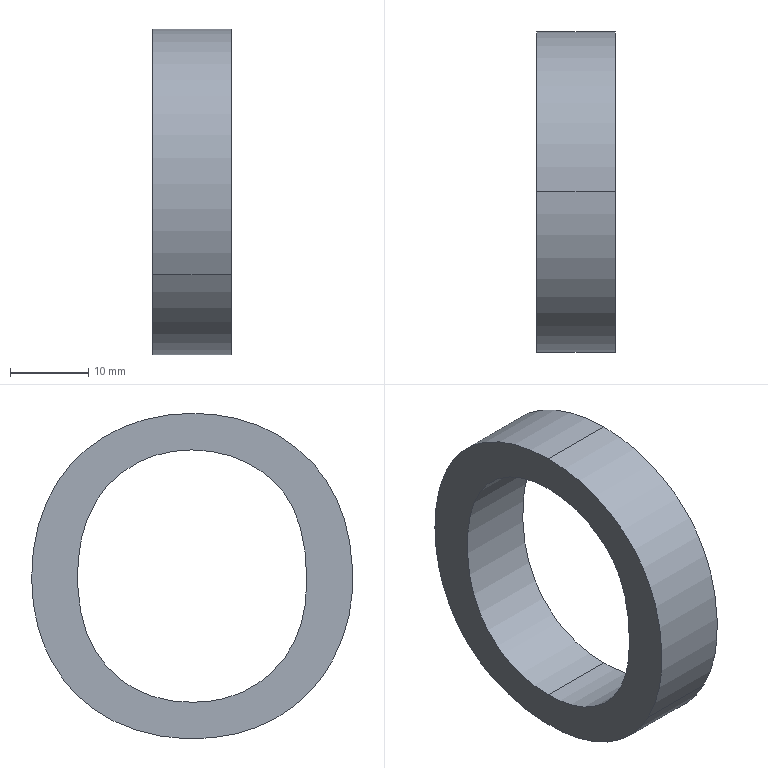Part | NX | features solid 2 | 1 solid | 8 faces | box 10 x 40.994 x 41.56 mm | volume 6055 mm3 | spline 6 | plane 2
STEP:
#1=CARTESIAN_POINT('',(2250.,-504.918,-666.115));
#2=VERTEX_POINT('',#1);
#3=CARTESIAN_POINT('',(2250.,-504.842,-633.885));
#4=VERTEX_POINT('',#3);
#5=CARTESIAN_POINT('',(2250.,-504.918,-666.115));
#6=CARTESIAN_POINT('',(2250.,-500.666,-666.145));
#7=CARTESIAN_POINT('',(2250.,-497.163,-664.769));
#8=CARTESIAN_POINT('',(2250.,-491.648,-659.163));
#9=CARTESIAN_POINT('',(2250.,-490.264,-655.193));
#10=CARTESIAN_POINT('',(2250.,-490.264,-646.826));
#11=CARTESIAN_POINT('',(2250.,-490.83,-643.981));
#12=CARTESIAN_POINT('',(2250.,-492.023,-641.557));
#13=CARTESIAN_POINT('',(2250.,-493.216,-639.132));
#14=CARTESIAN_POINT('',(2250.,-494.945,-637.266));
#15=CARTESIAN_POINT('',(2250.,-497.217,-635.918));
#16=CARTESIAN_POINT('',(2250.,-499.457,-634.589));
#17=CARTESIAN_POINT('',(2250.,-502.027,-633.916));
#18=CARTESIAN_POINT('',(2250.,-504.842,-633.885));
#19=B_SPLINE_CURVE_WITH_KNOTS('',3,(#5,#6,#7,#8,#9,#10,#11,#12,#13,#14,#15,#16,#17,#18),.UNSPECIFIED.,.F.,.F.,(4,2,2,3,3,4),(0.4029,0.5265,0.649,0.7248,0.8038,0.885),.UNSPECIFIED.);
#20=EDGE_CURVE('',#2,#4,#19,.T.);
#21=ORIENTED_EDGE('',*,*,#20,.F.);
#22=CARTESIAN_POINT('',(2260.,-504.918,-666.115));
#23=VERTEX_POINT('',#22);
#24=CARTESIAN_POINT('',(2260.,-504.918,-666.115));
#25=DIRECTION('',(-1.,0.,0.));
#26=VECTOR('',#25,1000.);
#27=LINE('',#24,#26);
#28=EDGE_CURVE('',#23,#2,#27,.T.);
#29=ORIENTED_EDGE('',*,*,#28,.F.);
#30=CARTESIAN_POINT('',(2260.,-504.842,-633.885));
#31=VERTEX_POINT('',#30);
#32=CARTESIAN_POINT('',(2260.,-504.918,-666.115));
#33=CARTESIAN_POINT('',(2260.,-500.666,-666.145));
#34=CARTESIAN_POINT('',(2260.,-497.163,-664.769));
#35=CARTESIAN_POINT('',(2260.,-491.648,-659.163));
#36=CARTESIAN_POINT('',(2260.,-490.264,-655.193));
#37=CARTESIAN_POINT('',(2260.,-490.264,-646.826));
#38=CARTESIAN_POINT('',(2260.,-490.83,-643.981));
#39=CARTESIAN_POINT('',(2260.,-492.023,-641.557));
#40=CARTESIAN_POINT('',(2260.,-493.216,-639.132));
#41=CARTESIAN_POINT('',(2260.,-494.945,-637.266));
#42=CARTESIAN_POINT('',(2260.,-497.217,-635.918));
#43=CARTESIAN_POINT('',(2260.,-499.457,-634.589));
#44=CARTESIAN_POINT('',(2260.,-502.027,-633.916));
#45=CARTESIAN_POINT('',(2260.,-504.842,-633.885));
#46=B_SPLINE_CURVE_WITH_KNOTS('',3,(#32,#33,#34,#35,#36,#37,#38,#39,#40,#41,#42,#43,#44,#45),.UNSPECIFIED.,.F.,.F.,(4,2,2,3,3,4),(0.4029,0.5265,0.649,0.7248,0.8038,0.885),.UNSPECIFIED.);
#47=EDGE_CURVE('',#23,#31,#46,.T.);
#48=ORIENTED_EDGE('',*,*,#47,.T.);
#49=CARTESIAN_POINT('',(2260.,-504.842,-633.885));
#50=DIRECTION('',(-1.,0.,0.));
#51=VECTOR('',#50,1000.);
#52=LINE('',#49,#51);
#53=EDGE_CURVE('',#31,#4,#52,.T.);
#54=ORIENTED_EDGE('',*,*,#53,.T.);
#55=EDGE_LOOP('',(#21,#29,#48,#54));
#56=FACE_BOUND('',#55,.T.);
#57=CARTESIAN_POINT('',(2260.,-504.918,-666.115));
#58=CARTESIAN_POINT('',(2250.,-504.918,-666.115));
#59=CARTESIAN_POINT('',(2260.,-502.844,-666.13));
#60=CARTESIAN_POINT('',(2250.,-502.844,-666.13));
#61=CARTESIAN_POINT('',(2260.,-499.063,-665.494));
#62=CARTESIAN_POINT('',(2250.,-499.063,-665.494));
#63=CARTESIAN_POINT('',(2260.,-495.169,-662.989));
#64=CARTESIAN_POINT('',(2250.,-495.169,-662.989));
#65=CARTESIAN_POINT('',(2260.,-492.683,-659.999));
#66=CARTESIAN_POINT('',(2250.,-492.683,-659.999));
#67=CARTESIAN_POINT('',(2260.,-491.36,-657.341));
#68=CARTESIAN_POINT('',(2250.,-491.36,-657.341));
#69=CARTESIAN_POINT('',(2260.,-490.523,-654.26));
#70=CARTESIAN_POINT('',(2250.,-490.523,-654.26));
#71=CARTESIAN_POINT('',(2260.,-490.187,-650.698));
#72=CARTESIAN_POINT('',(2250.,-490.187,-650.698));
#73=CARTESIAN_POINT('',(2260.,-490.359,-646.885));
#74=CARTESIAN_POINT('',(2250.,-490.359,-646.885));
#75=CARTESIAN_POINT('',(2260.,-491.091,-643.562));
#76=CARTESIAN_POINT('',(2250.,-491.091,-643.562));
#77=CARTESIAN_POINT('',(2260.,-492.412,-640.598));
#78=CARTESIAN_POINT('',(2250.,-492.412,-640.598));
#79=CARTESIAN_POINT('',(2260.,-494.719,-637.465));
#80=CARTESIAN_POINT('',(2250.,-494.719,-637.465));
#81=CARTESIAN_POINT('',(2260.,-498.874,-634.639));
#82=CARTESIAN_POINT('',(2250.,-498.874,-634.639));
#83=CARTESIAN_POINT('',(2260.,-502.752,-633.908));
#84=CARTESIAN_POINT('',(2250.,-502.752,-633.908));
#85=CARTESIAN_POINT('',(2260.,-504.842,-633.885));
#86=CARTESIAN_POINT('',(2250.,-504.842,-633.885));
#87=B_SPLINE_SURFACE_WITH_KNOTS('',3,1,((#57,#58),(#59,#60),(#61,#62),(#63,#64),(#65,#66),(#67,#68),(#69,#70),(#71,#72),(#73,#74),(#75,#76),(#77,#78),(#79,#80),(#81,#82),(#83,#84),(#85,#86)),.SURF_OF_LINEAR_EXTRUSION.,.F.,.F.,.F.,(4,1,1,1,1,1,1,1,1,1,1,1,4),(2,2),(0.4029,0.4632,0.5235,0.5536,0.5837,0.6138,0.644,0.6741,0.7042,0.7344,0.7645,0.8248,0.885),(0.,1.),.UNSPECIFIED.);
#88=ADVANCED_FACE('',(#56),#87,.T.);
#89=CARTESIAN_POINT('',(2250.,-515.191,-637.778));
#90=VERTEX_POINT('',#89);
#91=CARTESIAN_POINT('',(2250.,-504.842,-633.885));
#92=CARTESIAN_POINT('',(2250.,-508.849,-633.916));
#93=CARTESIAN_POINT('',(2250.,-512.291,-635.201));
#94=CARTESIAN_POINT('',(2250.,-515.191,-637.778));
#95=B_SPLINE_CURVE_WITH_KNOTS('',3,(#91,#92,#93,#94),.UNSPECIFIED.,.F.,.F.,(4,4),(0.885,1.),.PIECEWISE_BEZIER_KNOTS.);
#96=EDGE_CURVE('',#4,#90,#95,.T.);
#97=ORIENTED_EDGE('',*,*,#96,.F.);
#98=ORIENTED_EDGE('',*,*,#53,.F.);
#99=CARTESIAN_POINT('',(2260.,-515.191,-637.778));
#100=VERTEX_POINT('',#99);
#101=CARTESIAN_POINT('',(2260.,-504.842,-633.885));
#102=CARTESIAN_POINT('',(2260.,-508.849,-633.916));
#103=CARTESIAN_POINT('',(2260.,-512.291,-635.201));
#104=CARTESIAN_POINT('',(2260.,-515.191,-637.778));
#105=B_SPLINE_CURVE_WITH_KNOTS('',3,(#101,#102,#103,#104),.UNSPECIFIED.,.F.,.F.,(4,4),(0.885,1.),.PIECEWISE_BEZIER_KNOTS.);
#106=EDGE_CURVE('',#31,#100,#105,.T.);
#107=ORIENTED_EDGE('',*,*,#106,.T.);
#108=CARTESIAN_POINT('',(2260.,-515.191,-637.778));
#109=DIRECTION('',(-1.,0.,0.));
#110=VECTOR('',#109,1000.);
#111=LINE('',#108,#110);
#112=EDGE_CURVE('',#100,#90,#111,.T.);
#113=ORIENTED_EDGE('',*,*,#112,.T.);
#114=EDGE_LOOP('',(#97,#98,#107,#113));
#115=FACE_BOUND('',#114,.T.);
#116=CARTESIAN_POINT('',(2260.,-504.842,-633.885));
#117=CARTESIAN_POINT('',(2250.,-504.842,-633.885));
#118=CARTESIAN_POINT('',(2260.,-508.849,-633.916));
#119=CARTESIAN_POINT('',(2250.,-508.849,-633.916));
#120=CARTESIAN_POINT('',(2260.,-512.291,-635.201));
#121=CARTESIAN_POINT('',(2250.,-512.291,-635.201));
#122=CARTESIAN_POINT('',(2260.,-515.191,-637.778));
#123=CARTESIAN_POINT('',(2250.,-515.191,-637.778));
#124=B_SPLINE_SURFACE_WITH_KNOTS('',3,1,((#116,#117),(#118,#119),(#120,#121),(#122,#123)),.SURF_OF_LINEAR_EXTRUSION.,.F.,.F.,.F.,(4,4),(2,2),(0.885,1.),(0.,1.),.PIECEWISE_BEZIER_KNOTS.);
#125=ADVANCED_FACE('',(#115),#124,.T.);
#126=CARTESIAN_POINT('',(2250.,-522.928,-660.588));
#127=VERTEX_POINT('',#126);
#128=CARTESIAN_POINT('',(2250.,-504.872,-629.22));
#129=VERTEX_POINT('',#128);
#130=CARTESIAN_POINT('',(2250.,-522.928,-660.588));
#131=CARTESIAN_POINT('',(2250.,-524.559,-657.426));
#132=CARTESIAN_POINT('',(2250.,-525.4,-654.076));
#133=CARTESIAN_POINT('',(2250.,-525.4,-643.889));
#134=CARTESIAN_POINT('',(2250.,-523.488,-638.688));
#135=CARTESIAN_POINT('',(2250.,-515.855,-631.147));
#136=CARTESIAN_POINT('',(2250.,-510.914,-629.25));
#137=CARTESIAN_POINT('',(2250.,-504.872,-629.22));
#138=B_SPLINE_CURVE_WITH_KNOTS('',3,(#130,#131,#132,#133,#134,#135,#136,#137),.UNSPECIFIED.,.F.,.F.,(4,2,2,4),(0.,0.07116,0.2052,0.3386),.UNSPECIFIED.);
#139=EDGE_CURVE('',#127,#129,#138,.T.);
#140=ORIENTED_EDGE('',*,*,#139,.F.);
#141=CARTESIAN_POINT('',(2260.,-522.928,-660.588));
#142=VERTEX_POINT('',#141);
#143=CARTESIAN_POINT('',(2260.,-522.928,-660.588));
#144=DIRECTION('',(-1.,0.,0.));
#145=VECTOR('',#144,1000.);
#146=LINE('',#143,#145);
#147=EDGE_CURVE('',#142,#127,#146,.T.);
#148=ORIENTED_EDGE('',*,*,#147,.F.);
#149=CARTESIAN_POINT('',(2260.,-504.872,-629.22));
#150=VERTEX_POINT('',#149);
#151=CARTESIAN_POINT('',(2260.,-522.928,-660.588));
#152=CARTESIAN_POINT('',(2260.,-524.559,-657.426));
#153=CARTESIAN_POINT('',(2260.,-525.4,-654.076));
#154=CARTESIAN_POINT('',(2260.,-525.4,-643.889));
#155=CARTESIAN_POINT('',(2260.,-523.488,-638.688));
#156=CARTESIAN_POINT('',(2260.,-515.855,-631.147));
#157=CARTESIAN_POINT('',(2260.,-510.914,-629.25));
#158=CARTESIAN_POINT('',(2260.,-504.872,-629.22));
#159=B_SPLINE_CURVE_WITH_KNOTS('',3,(#151,#152,#153,#154,#155,#156,#157,#158),.UNSPECIFIED.,.F.,.F.,(4,2,2,4),(0.,0.07116,0.2052,0.3386),.UNSPECIFIED.);
#160=EDGE_CURVE('',#142,#150,#159,.T.);
#161=ORIENTED_EDGE('',*,*,#160,.T.);
#162=CARTESIAN_POINT('',(2260.,-504.872,-629.22));
#163=DIRECTION('',(-1.,0.,0.));
#164=VECTOR('',#163,1000.);
#165=LINE('',#162,#164);
#166=EDGE_CURVE('',#150,#129,#165,.T.);
#167=ORIENTED_EDGE('',*,*,#166,.T.);
#168=EDGE_LOOP('',(#140,#148,#161,#167));
#169=FACE_BOUND('',#168,.T.);
#170=CARTESIAN_POINT('',(2260.,-522.928,-660.588));
#171=CARTESIAN_POINT('',(2250.,-522.928,-660.588));
#172=CARTESIAN_POINT('',(2260.,-523.898,-658.707));
#173=CARTESIAN_POINT('',(2250.,-523.898,-658.707));
#174=CARTESIAN_POINT('',(2260.,-524.934,-655.787));
#175=CARTESIAN_POINT('',(2250.,-524.934,-655.787));
#176=CARTESIAN_POINT('',(2260.,-525.444,-651.693));
#177=CARTESIAN_POINT('',(2250.,-525.444,-651.693));
#178=CARTESIAN_POINT('',(2260.,-525.368,-647.482));
#179=CARTESIAN_POINT('',(2250.,-525.368,-647.482));
#180=CARTESIAN_POINT('',(2260.,-524.594,-642.841));
#181=CARTESIAN_POINT('',(2250.,-524.594,-642.841));
#182=CARTESIAN_POINT('',(2260.,-522.526,-638.112));
#183=CARTESIAN_POINT('',(2250.,-522.526,-638.112));
#184=CARTESIAN_POINT('',(2260.,-519.235,-634.2));
#185=CARTESIAN_POINT('',(2250.,-519.235,-634.2));
#186=CARTESIAN_POINT('',(2260.,-513.777,-630.387));
#187=CARTESIAN_POINT('',(2250.,-513.777,-630.387));
#188=CARTESIAN_POINT('',(2260.,-508.705,-629.239));
#189=CARTESIAN_POINT('',(2250.,-508.705,-629.239));
#190=CARTESIAN_POINT('',(2260.,-504.872,-629.22));
#191=CARTESIAN_POINT('',(2250.,-504.872,-629.22));
#192=B_SPLINE_SURFACE_WITH_KNOTS('',3,1,((#170,#171),(#172,#173),(#174,#175),(#176,#177),(#178,#179),(#180,#181),(#182,#183),(#184,#185),(#186,#187),(#188,#189),(#190,#191)),.SURF_OF_LINEAR_EXTRUSION.,.F.,.F.,.F.,(4,1,1,1,1,1,1,1,4),(2,2),(0.,0.04233,0.06349,0.08466,0.127,0.1693,0.2116,0.254,0.3386),(0.,1.),.UNSPECIFIED.);
#193=ADVANCED_FACE('',(#169),#192,.T.);
#194=CARTESIAN_POINT('',(2250.,-487.052,-661.021));
#195=VERTEX_POINT('',#194);
#196=CARTESIAN_POINT('',(2250.,-504.872,-629.22));
#197=CARTESIAN_POINT('',(2250.,-500.895,-629.25));
#198=CARTESIAN_POINT('',(2250.,-497.346,-630.153));
#199=CARTESIAN_POINT('',(2250.,-494.188,-631.911));
#200=CARTESIAN_POINT('',(2250.,-490.998,-633.686));
#201=CARTESIAN_POINT('',(2250.,-488.582,-636.164));
#202=CARTESIAN_POINT('',(2250.,-485.247,-642.497));
#203=CARTESIAN_POINT('',(2250.,-484.406,-646.092));
#204=CARTESIAN_POINT('',(2250.,-484.406,-654.184));
#205=CARTESIAN_POINT('',(2250.,-485.262,-657.824));
#206=CARTESIAN_POINT('',(2250.,-487.052,-661.021));
#207=B_SPLINE_CURVE_WITH_KNOTS('',3,(#196,#197,#198,#199,#200,#201,#202,#203,#204,#205,#206),.UNSPECIFIED.,.F.,.F.,(4,3,2,2,4),(0.3386,0.4247,0.5061,0.5876,0.6712),.UNSPECIFIED.);
#208=EDGE_CURVE('',#129,#195,#207,.T.);
#209=ORIENTED_EDGE('',*,*,#208,.F.);
#210=ORIENTED_EDGE('',*,*,#166,.F.);
#211=CARTESIAN_POINT('',(2260.,-487.052,-661.021));
#212=VERTEX_POINT('',#211);
#213=CARTESIAN_POINT('',(2260.,-504.872,-629.22));
#214=CARTESIAN_POINT('',(2260.,-500.895,-629.25));
#215=CARTESIAN_POINT('',(2260.,-497.346,-630.153));
#216=CARTESIAN_POINT('',(2260.,-494.188,-631.911));
#217=CARTESIAN_POINT('',(2260.,-490.998,-633.686));
#218=CARTESIAN_POINT('',(2260.,-488.582,-636.164));
#219=CARTESIAN_POINT('',(2260.,-485.247,-642.497));
#220=CARTESIAN_POINT('',(2260.,-484.406,-646.092));
#221=CARTESIAN_POINT('',(2260.,-484.406,-654.184));
#222=CARTESIAN_POINT('',(2260.,-485.262,-657.824));
#223=CARTESIAN_POINT('',(2260.,-487.052,-661.021));
#224=B_SPLINE_CURVE_WITH_KNOTS('',3,(#213,#214,#215,#216,#217,#218,#219,#220,#221,#222,#223),.UNSPECIFIED.,.F.,.F.,(4,3,2,2,4),(0.3386,0.4247,0.5061,0.5876,0.6712),.UNSPECIFIED.);
#225=EDGE_CURVE('',#150,#212,#224,.T.);
#226=ORIENTED_EDGE('',*,*,#225,.T.);
#227=CARTESIAN_POINT('',(2260.,-487.052,-661.021));
#228=DIRECTION('',(-1.,0.,0.));
#229=VECTOR('',#228,1000.);
#230=LINE('',#227,#229);
#231=EDGE_CURVE('',#212,#195,#230,.T.);
#232=ORIENTED_EDGE('',*,*,#231,.T.);
#233=EDGE_LOOP('',(#209,#210,#226,#232));
#234=FACE_BOUND('',#233,.T.);
#235=CARTESIAN_POINT('',(2260.,-504.872,-629.22));
#236=CARTESIAN_POINT('',(2250.,-504.872,-629.22));
#237=CARTESIAN_POINT('',(2260.,-502.951,-629.235));
#238=CARTESIAN_POINT('',(2250.,-502.951,-629.235));
#239=CARTESIAN_POINT('',(2260.,-500.223,-629.559));
#240=CARTESIAN_POINT('',(2250.,-500.223,-629.559));
#241=CARTESIAN_POINT('',(2260.,-496.855,-630.609));
#242=CARTESIAN_POINT('',(2250.,-496.855,-630.609));
#243=CARTESIAN_POINT('',(2260.,-494.514,-631.667));
#244=CARTESIAN_POINT('',(2250.,-494.514,-631.667));
#245=CARTESIAN_POINT('',(2260.,-492.139,-633.14));
#246=CARTESIAN_POINT('',(2250.,-492.139,-633.14));
#247=CARTESIAN_POINT('',(2260.,-489.444,-635.44));
#248=CARTESIAN_POINT('',(2250.,-489.444,-635.44));
#249=CARTESIAN_POINT('',(2260.,-486.783,-639.041));
#250=CARTESIAN_POINT('',(2250.,-486.783,-639.041));
#251=CARTESIAN_POINT('',(2260.,-485.152,-643.391));
#252=CARTESIAN_POINT('',(2250.,-485.152,-643.391));
#253=CARTESIAN_POINT('',(2260.,-484.508,-647.139));
#254=CARTESIAN_POINT('',(2250.,-484.508,-647.139));
#255=CARTESIAN_POINT('',(2260.,-484.352,-650.16));
#256=CARTESIAN_POINT('',(2250.,-484.352,-650.16));
#257=CARTESIAN_POINT('',(2260.,-484.519,-653.158));
#258=CARTESIAN_POINT('',(2250.,-484.519,-653.158));
#259=CARTESIAN_POINT('',(2260.,-485.174,-656.88));
#260=CARTESIAN_POINT('',(2250.,-485.174,-656.88));
#261=CARTESIAN_POINT('',(2260.,-486.162,-659.432));
#262=CARTESIAN_POINT('',(2250.,-486.162,-659.432));
#263=CARTESIAN_POINT('',(2260.,-487.052,-661.021));
#264=CARTESIAN_POINT('',(2250.,-487.052,-661.021));
#265=B_SPLINE_SURFACE_WITH_KNOTS('',3,1,((#235,#236),(#237,#238),(#239,#240),(#241,#242),(#243,#244),(#245,#246),(#247,#248),(#249,#250),(#251,#252),(#253,#254),(#255,#256),(#257,#258),(#259,#260),(#261,#262),(#263,#264)),.SURF_OF_LINEAR_EXTRUSION.,.F.,.F.,.F.,(4,1,1,1,1,1,1,1,1,1,1,1,4),(2,2),(0.3386,0.3802,0.401,0.4218,0.4426,0.4634,0.5049,0.5465,0.5673,0.5881,0.6089,0.6296,0.6712),(0.,1.),.UNSPECIFIED.);
#266=ADVANCED_FACE('',(#234),#265,.T.);
#267=CARTESIAN_POINT('',(2250.,-487.052,-661.021));
#268=CARTESIAN_POINT('',(2250.,-488.796,-664.249));
#269=CARTESIAN_POINT('',(2250.,-491.274,-666.681));
#270=CARTESIAN_POINT('',(2250.,-497.717,-669.979));
#271=CARTESIAN_POINT('',(2250.,-501.186,-670.78));
#272=CARTESIAN_POINT('',(2250.,-508.926,-670.78));
#273=CARTESIAN_POINT('',(2250.,-512.536,-669.908));
#274=CARTESIAN_POINT('',(2250.,-515.729,-668.077));
#275=CARTESIAN_POINT('',(2250.,-518.884,-666.268));
#276=CARTESIAN_POINT('',(2250.,-521.285,-663.774));
#277=CARTESIAN_POINT('',(2250.,-522.928,-660.588));
#278=B_SPLINE_CURVE_WITH_KNOTS('',3,(#267,#268,#269,#270,#271,#272,#273,#274,#275,#276,#277),.UNSPECIFIED.,.F.,.F.,(4,2,2,3,4),(0.6712,0.752,0.8326,0.9197,1.),.UNSPECIFIED.);
#279=EDGE_CURVE('',#195,#127,#278,.T.);
#280=ORIENTED_EDGE('',*,*,#279,.F.);
#281=ORIENTED_EDGE('',*,*,#231,.F.);
#282=CARTESIAN_POINT('',(2260.,-487.052,-661.021));
#283=CARTESIAN_POINT('',(2260.,-488.796,-664.249));
#284=CARTESIAN_POINT('',(2260.,-491.274,-666.681));
#285=CARTESIAN_POINT('',(2260.,-497.717,-669.979));
#286=CARTESIAN_POINT('',(2260.,-501.186,-670.78));
#287=CARTESIAN_POINT('',(2260.,-508.926,-670.78));
#288=CARTESIAN_POINT('',(2260.,-512.536,-669.908));
#289=CARTESIAN_POINT('',(2260.,-515.729,-668.077));
#290=CARTESIAN_POINT('',(2260.,-518.884,-666.268));
#291=CARTESIAN_POINT('',(2260.,-521.285,-663.774));
#292=CARTESIAN_POINT('',(2260.,-522.928,-660.588));
#293=B_SPLINE_CURVE_WITH_KNOTS('',3,(#282,#283,#284,#285,#286,#287,#288,#289,#290,#291,#292),.UNSPECIFIED.,.F.,.F.,(4,2,2,3,4),(0.6712,0.752,0.8326,0.9197,1.),.UNSPECIFIED.);
#294=EDGE_CURVE('',#212,#142,#293,.T.);
#295=ORIENTED_EDGE('',*,*,#294,.T.);
#296=ORIENTED_EDGE('',*,*,#147,.T.);
#297=EDGE_LOOP('',(#280,#281,#295,#296));
#298=FACE_BOUND('',#297,.T.);
#299=CARTESIAN_POINT('',(2260.,-487.052,-661.021));
#300=CARTESIAN_POINT('',(2250.,-487.052,-661.021));
#301=CARTESIAN_POINT('',(2260.,-487.939,-662.662));
#302=CARTESIAN_POINT('',(2250.,-487.939,-662.662));
#303=CARTESIAN_POINT('',(2260.,-490.072,-665.53));
#304=CARTESIAN_POINT('',(2250.,-490.072,-665.53));
#305=CARTESIAN_POINT('',(2260.,-494.539,-668.627));
#306=CARTESIAN_POINT('',(2250.,-494.539,-668.627));
#307=CARTESIAN_POINT('',(2260.,-498.889,-670.15));
#308=CARTESIAN_POINT('',(2250.,-498.889,-670.15));
#309=CARTESIAN_POINT('',(2260.,-502.487,-670.719));
#310=CARTESIAN_POINT('',(2250.,-502.487,-670.719));
#311=CARTESIAN_POINT('',(2260.,-506.287,-670.861));
#312=CARTESIAN_POINT('',(2250.,-506.287,-670.861));
#313=CARTESIAN_POINT('',(2260.,-509.89,-670.417));
#314=CARTESIAN_POINT('',(2250.,-509.89,-670.417));
#315=CARTESIAN_POINT('',(2260.,-513.206,-669.351));
#316=CARTESIAN_POINT('',(2250.,-513.206,-669.351));
#317=CARTESIAN_POINT('',(2260.,-515.506,-668.272));
#318=CARTESIAN_POINT('',(2250.,-515.506,-668.272));
#319=CARTESIAN_POINT('',(2260.,-517.863,-666.747));
#320=CARTESIAN_POINT('',(2250.,-517.863,-666.747));
#321=CARTESIAN_POINT('',(2260.,-520.52,-664.398));
#322=CARTESIAN_POINT('',(2250.,-520.52,-664.398));
#323=CARTESIAN_POINT('',(2260.,-522.087,-662.22));
#324=CARTESIAN_POINT('',(2250.,-522.087,-662.22));
#325=CARTESIAN_POINT('',(2260.,-522.928,-660.588));
#326=CARTESIAN_POINT('',(2250.,-522.928,-660.588));
#327=B_SPLINE_SURFACE_WITH_KNOTS('',3,1,((#299,#300),(#301,#302),(#303,#304),(#305,#306),(#307,#308),(#309,#310),(#311,#312),(#313,#314),(#315,#316),(#317,#318),(#319,#320),(#321,#322),(#323,#324),(#325,#326)),.SURF_OF_LINEAR_EXTRUSION.,.F.,.F.,.F.,(4,1,1,1,1,1,1,1,1,1,1,4),(2,2),(0.6712,0.7123,0.7534,0.7945,0.8151,0.8356,0.8767,0.8973,0.9178,0.9384,0.9589,1.),(0.,1.),.UNSPECIFIED.);
#328=ADVANCED_FACE('',(#298),#327,.T.);
#329=CARTESIAN_POINT('',(2250.,-515.191,-637.778));
#330=CARTESIAN_POINT('',(2250.,-518.073,-640.34));
#331=CARTESIAN_POINT('',(2250.,-519.541,-644.639));
#332=CARTESIAN_POINT('',(2250.,-519.541,-655.438));
#333=CARTESIAN_POINT('',(2250.,-518.15,-659.231));
#334=CARTESIAN_POINT('',(2250.,-512.612,-664.769));
#335=CARTESIAN_POINT('',(2250.,-509.109,-666.145));
#336=CARTESIAN_POINT('',(2250.,-504.918,-666.115));
#337=B_SPLINE_CURVE_WITH_KNOTS('',3,(#329,#330,#331,#332,#333,#334,#335,#336),.UNSPECIFIED.,.F.,.F.,(4,2,2,4),(0.,0.1538,0.2784,0.4029),.UNSPECIFIED.);
#338=EDGE_CURVE('',#90,#2,#337,.T.);
#339=ORIENTED_EDGE('',*,*,#338,.F.);
#340=ORIENTED_EDGE('',*,*,#112,.F.);
#341=CARTESIAN_POINT('',(2260.,-515.191,-637.778));
#342=CARTESIAN_POINT('',(2260.,-518.073,-640.34));
#343=CARTESIAN_POINT('',(2260.,-519.541,-644.639));
#344=CARTESIAN_POINT('',(2260.,-519.541,-655.438));
#345=CARTESIAN_POINT('',(2260.,-518.15,-659.231));
#346=CARTESIAN_POINT('',(2260.,-512.612,-664.769));
#347=CARTESIAN_POINT('',(2260.,-509.109,-666.145));
#348=CARTESIAN_POINT('',(2260.,-504.918,-666.115));
#349=B_SPLINE_CURVE_WITH_KNOTS('',3,(#341,#342,#343,#344,#345,#346,#347,#348),.UNSPECIFIED.,.F.,.F.,(4,2,2,4),(0.,0.1538,0.2784,0.4029),.UNSPECIFIED.);
#350=EDGE_CURVE('',#100,#23,#349,.T.);
#351=ORIENTED_EDGE('',*,*,#350,.T.);
#352=ORIENTED_EDGE('',*,*,#28,.T.);
#353=EDGE_LOOP('',(#339,#340,#351,#352));
#354=FACE_BOUND('',#353,.T.);
#355=CARTESIAN_POINT('',(2260.,-515.191,-637.778));
#356=CARTESIAN_POINT('',(2250.,-515.191,-637.778));
#357=CARTESIAN_POINT('',(2260.,-516.135,-638.617));
#358=CARTESIAN_POINT('',(2250.,-516.135,-638.617));
#359=CARTESIAN_POINT('',(2260.,-517.719,-640.667));
#360=CARTESIAN_POINT('',(2250.,-517.719,-640.667));
#361=CARTESIAN_POINT('',(2260.,-518.934,-644.156));
#362=CARTESIAN_POINT('',(2250.,-518.934,-644.156));
#363=CARTESIAN_POINT('',(2260.,-519.435,-647.475));
#364=CARTESIAN_POINT('',(2250.,-519.435,-647.475));
#365=CARTESIAN_POINT('',(2260.,-519.585,-650.28));
#366=CARTESIAN_POINT('',(2250.,-519.585,-650.28));
#367=CARTESIAN_POINT('',(2260.,-519.465,-653.181));
#368=CARTESIAN_POINT('',(2250.,-519.465,-653.181));
#369=CARTESIAN_POINT('',(2260.,-518.825,-656.594));
#370=CARTESIAN_POINT('',(2250.,-518.825,-656.594));
#371=CARTESIAN_POINT('',(2260.,-517.199,-660.257));
#372=CARTESIAN_POINT('',(2250.,-517.199,-660.257));
#373=CARTESIAN_POINT('',(2260.,-512.698,-664.804));
#374=CARTESIAN_POINT('',(2250.,-512.698,-664.804));
#375=CARTESIAN_POINT('',(2260.,-508.307,-666.139));
#376=CARTESIAN_POINT('',(2250.,-508.307,-666.139));
#377=CARTESIAN_POINT('',(2260.,-504.918,-666.115));
#378=CARTESIAN_POINT('',(2250.,-504.918,-666.115));
#379=B_SPLINE_SURFACE_WITH_KNOTS('',3,1,((#355,#356),(#357,#358),(#359,#360),(#361,#362),(#363,#364),(#365,#366),(#367,#368),(#369,#370),(#371,#372),(#373,#374),(#375,#376),(#377,#378)),.SURF_OF_LINEAR_EXTRUSION.,.F.,.F.,.F.,(4,1,1,1,1,1,1,1,1,4),(2,2),(0.,0.05037,0.1007,0.1259,0.1511,0.1763,0.2015,0.2518,0.3022,0.4029),(0.,1.),.UNSPECIFIED.);
#380=ADVANCED_FACE('',(#354),#379,.T.);
#381=ORIENTED_EDGE('',*,*,#160,.F.);
#382=ORIENTED_EDGE('',*,*,#294,.F.);
#383=ORIENTED_EDGE('',*,*,#225,.F.);
#384=EDGE_LOOP('',(#381,#382,#383));
#385=FACE_BOUND('',#384,.T.);
#386=ORIENTED_EDGE('',*,*,#47,.F.);
#387=ORIENTED_EDGE('',*,*,#350,.F.);
#388=ORIENTED_EDGE('',*,*,#106,.F.);
#389=EDGE_LOOP('',(#386,#387,#388));
#390=FACE_BOUND('',#389,.T.);
#391=CARTESIAN_POINT('',(2260.,-522.322,-638.249));
#392=DIRECTION('',(1.,0.,0.));
#393=DIRECTION('',(0.,1.,0.));
#394=AXIS2_PLACEMENT_3D('',#391,#392,#393);
#395=PLANE('',#394);
#396=ADVANCED_FACE('',(#385,#390),#395,.T.);
#397=ORIENTED_EDGE('',*,*,#139,.T.);
#398=ORIENTED_EDGE('',*,*,#208,.T.);
#399=ORIENTED_EDGE('',*,*,#279,.T.);
#400=EDGE_LOOP('',(#397,#398,#399));
#401=FACE_BOUND('',#400,.T.);
#402=ORIENTED_EDGE('',*,*,#20,.T.);
#403=ORIENTED_EDGE('',*,*,#96,.T.);
#404=ORIENTED_EDGE('',*,*,#338,.T.);
#405=EDGE_LOOP('',(#402,#403,#404));
#406=FACE_BOUND('',#405,.T.);
#407=CARTESIAN_POINT('',(2250.,-522.322,-638.249));
#408=DIRECTION('',(1.,0.,0.));
#409=DIRECTION('',(0.,1.,0.));
#410=AXIS2_PLACEMENT_3D('',#407,#408,#409);
#411=PLANE('',#410);
#412=ADVANCED_FACE('',(#401,#406),#411,.F.);
#413=CLOSED_SHELL('',(#88,#125,#193,#266,#328,#380,#396,#412));
#414=MANIFOLD_SOLID_BREP('',#413);
#415=(LENGTH_UNIT()NAMED_UNIT(*)SI_UNIT(.MILLI.,.METRE.));
#416=UNCERTAINTY_MEASURE_WITH_UNIT(LENGTH_MEASURE(0.0508),#415,'','');
#417=(NAMED_UNIT(*)PLANE_ANGLE_UNIT()SI_UNIT($,.RADIAN.));
#418=(NAMED_UNIT(*)SI_UNIT($,.STERADIAN.)SOLID_ANGLE_UNIT());
#419=(GEOMETRIC_REPRESENTATION_CONTEXT(3)GLOBAL_UNCERTAINTY_ASSIGNED_CONTEXT((#416))GLOBAL_UNIT_ASSIGNED_CONTEXT((#415,#417,#418))REPRESENTATION_CONTEXT('',''));
#420=ADVANCED_BREP_SHAPE_REPRESENTATION('',(#414),#419);